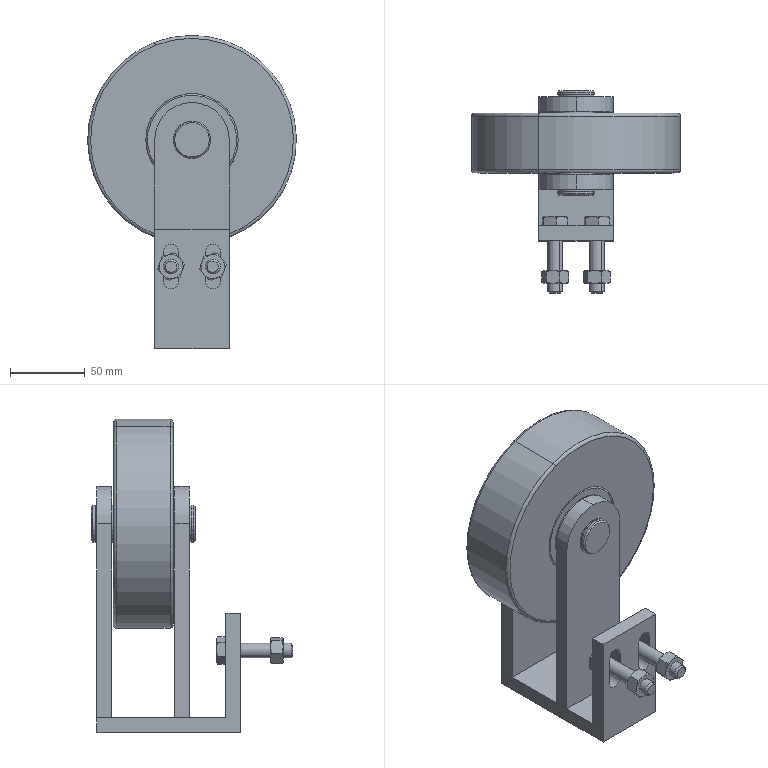Part | SolidWorks | features ReferencePattern 2, LocalLPattern 1 | 14 solids | 396 faces | box 140 x 135.4 x 210 mm | volume 1382662 mm3 | torus 112 | cylinder 90 | plane 90 | cone 52 | sphere 52 | commonest cylinder face diameters 25 x26 10 x12 23.9 x12 37.333 x8 62 x8 14.4 x4